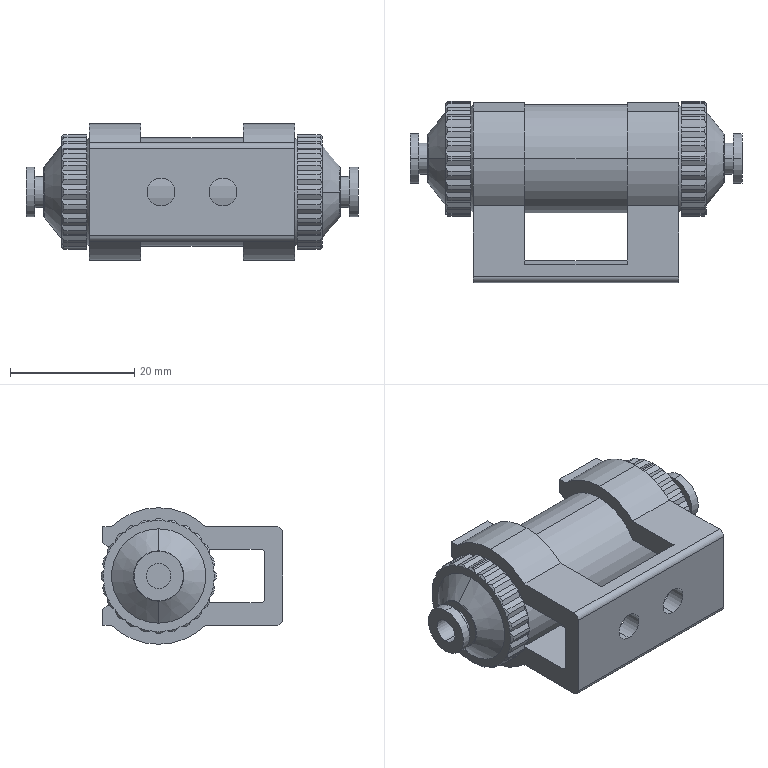Part | STEP file | Vacuum filter Qilike VFD-02-04-1 | 1 solid | 278 faces | box 53.5 x 29.25 x 22 mm | volume 14857 mm3 | plane 138 | cylinder 78 | cone 58 | spline 4 | commonest cylinder face diameters 18.5 x50 22 x6 4 x4 4.5 x4 5 x4 8 x4